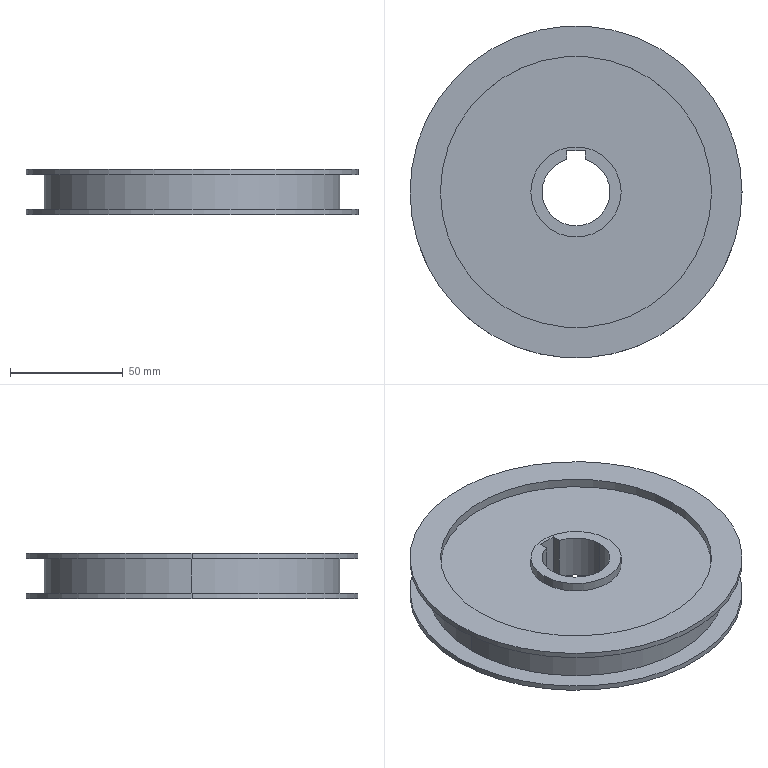Part | STEP file | Pulley 150 belt ha13v1V11 | 1 solid | 28 faces | box 147 x 147 x 20 mm | volume 190388 mm3 | cylinder 17 | plane 11 | commonest cylinder face diameters 40 x4 120 x4 147 x4 30 x3 131 x2